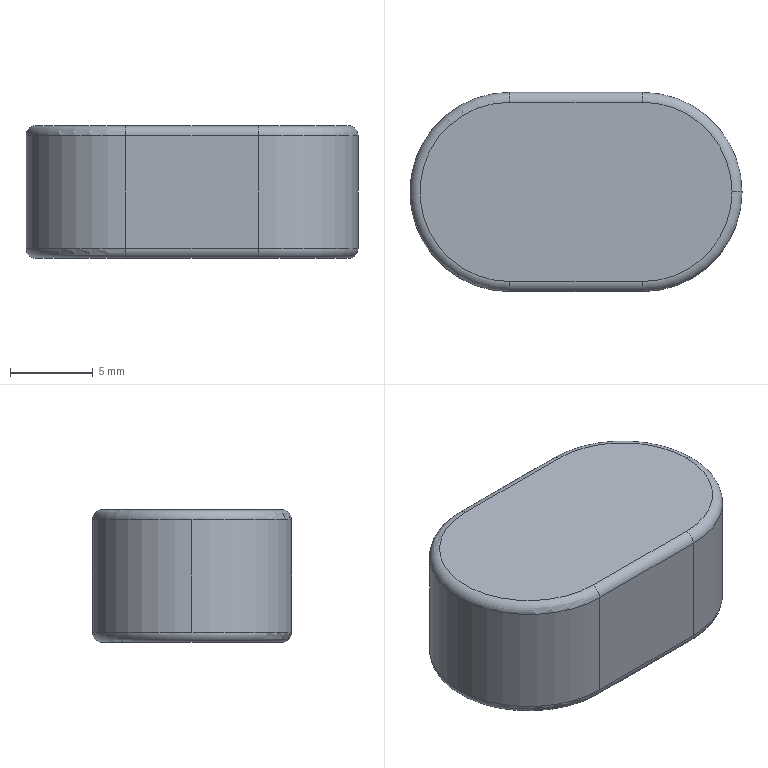Part | SolidWorks | features Extrusion 1, Fillet 1 | 1 solid | 17 faces | box 20 x 12 x 8 mm | volume 1665 mm3 | cylinder 7 | torus 6 | plane 4 | commonest cylinder face diameters 1.2 x4 12 x3
STEP:
#1=CARTESIAN_POINT('',(9.4,0.,0.));
#2=VERTEX_POINT('',#1);
#3=CARTESIAN_POINT('',(4.,-5.4,0.));
#4=VERTEX_POINT('',#3);
#5=CARTESIAN_POINT('',(4.,0.,0.));
#6=DIRECTION('',(0.,0.,-1.));
#7=DIRECTION('',(1.,0.,0.));
#8=AXIS2_PLACEMENT_3D('',#5,#6,#7);
#9=CIRCLE('',#8,5.4);
#10=EDGE_CURVE('',#2,#4,#9,.T.);
#11=ORIENTED_EDGE('',*,*,#10,.F.);
#12=CARTESIAN_POINT('',(10.,0.,0.6));
#13=VERTEX_POINT('',#12);
#14=CARTESIAN_POINT('',(9.4,0.,0.6));
#15=DIRECTION('',(0.,-1.,0.));
#16=DIRECTION('',(0.,0.,-1.));
#17=AXIS2_PLACEMENT_3D('',#14,#15,#16);
#18=CIRCLE('',#17,0.6);
#19=EDGE_CURVE('',#2,#13,#18,.T.);
#20=ORIENTED_EDGE('',*,*,#19,.T.);
#21=CARTESIAN_POINT('',(4.,-6.,0.6));
#22=VERTEX_POINT('',#21);
#23=CARTESIAN_POINT('',(4.,0.,0.6));
#24=DIRECTION('',(0.,0.,1.));
#25=DIRECTION('',(1.,0.,0.));
#26=AXIS2_PLACEMENT_3D('',#23,#24,#25);
#27=CIRCLE('',#26,6.);
#28=EDGE_CURVE('',#22,#13,#27,.T.);
#29=ORIENTED_EDGE('',*,*,#28,.F.);
#30=CARTESIAN_POINT('',(4.,-5.4,0.6));
#31=DIRECTION('',(1.,0.,0.));
#32=DIRECTION('',(0.,0.,-1.));
#33=AXIS2_PLACEMENT_3D('',#30,#31,#32);
#34=CIRCLE('',#33,0.6);
#35=EDGE_CURVE('',#22,#4,#34,.T.);
#36=ORIENTED_EDGE('',*,*,#35,.T.);
#37=EDGE_LOOP('',(#11,#20,#29,#36));
#38=FACE_OUTER_BOUND('',#37,.T.);
#39=CARTESIAN_POINT('',(4.,0.,0.6));
#40=DIRECTION('',(0.,0.,1.));
#41=DIRECTION('',(1.,0.,0.));
#42=AXIS2_PLACEMENT_3D('',#39,#40,#41);
#43=TOROIDAL_SURFACE('',#42,5.4,0.6);
#44=ADVANCED_FACE('',(#38),#43,.T.);
#45=CARTESIAN_POINT('',(10.,0.,7.4));
#46=VERTEX_POINT('',#45);
#47=CARTESIAN_POINT('',(4.,-6.,7.4));
#48=VERTEX_POINT('',#47);
#49=CARTESIAN_POINT('',(4.,0.,7.4));
#50=DIRECTION('',(0.,0.,-1.));
#51=DIRECTION('',(1.,0.,0.));
#52=AXIS2_PLACEMENT_3D('',#49,#50,#51);
#53=CIRCLE('',#52,6.);
#54=EDGE_CURVE('',#46,#48,#53,.T.);
#55=ORIENTED_EDGE('',*,*,#54,.F.);
#56=CARTESIAN_POINT('',(9.4,0.,8.));
#57=VERTEX_POINT('',#56);
#58=CARTESIAN_POINT('',(9.4,0.,7.4));
#59=DIRECTION('',(0.,-1.,0.));
#60=DIRECTION('',(0.,0.,-1.));
#61=AXIS2_PLACEMENT_3D('',#58,#59,#60);
#62=CIRCLE('',#61,0.6);
#63=EDGE_CURVE('',#46,#57,#62,.T.);
#64=ORIENTED_EDGE('',*,*,#63,.T.);
#65=CARTESIAN_POINT('',(4.,-5.4,8.));
#66=VERTEX_POINT('',#65);
#67=CARTESIAN_POINT('',(4.,0.,8.));
#68=DIRECTION('',(0.,0.,1.));
#69=DIRECTION('',(1.,0.,0.));
#70=AXIS2_PLACEMENT_3D('',#67,#68,#69);
#71=CIRCLE('',#70,5.4);
#72=EDGE_CURVE('',#66,#57,#71,.T.);
#73=ORIENTED_EDGE('',*,*,#72,.F.);
#74=CARTESIAN_POINT('',(4.,-5.4,7.4));
#75=DIRECTION('',(1.,0.,0.));
#76=DIRECTION('',(0.,0.,-1.));
#77=AXIS2_PLACEMENT_3D('',#74,#75,#76);
#78=CIRCLE('',#77,0.6);
#79=EDGE_CURVE('',#66,#48,#78,.T.);
#80=ORIENTED_EDGE('',*,*,#79,.T.);
#81=EDGE_LOOP('',(#55,#64,#73,#80));
#82=FACE_OUTER_BOUND('',#81,.T.);
#83=CARTESIAN_POINT('',(4.,0.,7.4));
#84=DIRECTION('',(0.,0.,1.));
#85=DIRECTION('',(1.,0.,0.));
#86=AXIS2_PLACEMENT_3D('',#83,#84,#85);
#87=TOROIDAL_SURFACE('',#86,5.4,0.6);
#88=ADVANCED_FACE('',(#82),#87,.T.);
#89=CARTESIAN_POINT('',(-4.,-6.,7.4));
#90=VERTEX_POINT('',#89);
#91=CARTESIAN_POINT('',(-10.,0.,7.4));
#92=VERTEX_POINT('',#91);
#93=CARTESIAN_POINT('',(-4.,0.,7.4));
#94=DIRECTION('',(0.,0.,-1.));
#95=DIRECTION('',(1.,0.,0.));
#96=AXIS2_PLACEMENT_3D('',#93,#94,#95);
#97=CIRCLE('',#96,6.);
#98=EDGE_CURVE('',#90,#92,#97,.T.);
#99=ORIENTED_EDGE('',*,*,#98,.T.);
#100=CARTESIAN_POINT('',(-10.,0.,0.6));
#101=VERTEX_POINT('',#100);
#102=CARTESIAN_POINT('',(-10.,0.,8.));
#103=DIRECTION('',(0.,0.,-1.));
#104=VECTOR('',#103,1000.);
#105=LINE('',#102,#104);
#106=EDGE_CURVE('',#92,#101,#105,.T.);
#107=ORIENTED_EDGE('',*,*,#106,.T.);
#108=CARTESIAN_POINT('',(-4.,-6.,0.6));
#109=VERTEX_POINT('',#108);
#110=CARTESIAN_POINT('',(-4.,0.,0.6));
#111=DIRECTION('',(0.,0.,1.));
#112=DIRECTION('',(1.,0.,0.));
#113=AXIS2_PLACEMENT_3D('',#110,#111,#112);
#114=CIRCLE('',#113,6.);
#115=EDGE_CURVE('',#101,#109,#114,.T.);
#116=ORIENTED_EDGE('',*,*,#115,.T.);
#117=CARTESIAN_POINT('',(-4.,-6.,8.));
#118=DIRECTION('',(0.,0.,-1.));
#119=VECTOR('',#118,1000.);
#120=LINE('',#117,#119);
#121=EDGE_CURVE('',#90,#109,#120,.T.);
#122=ORIENTED_EDGE('',*,*,#121,.F.);
#123=EDGE_LOOP('',(#99,#107,#116,#122));
#124=FACE_OUTER_BOUND('',#123,.T.);
#125=CARTESIAN_POINT('',(-4.,0.,8.));
#126=DIRECTION('',(0.,0.,-1.));
#127=DIRECTION('',(-1.,0.,0.));
#128=AXIS2_PLACEMENT_3D('',#125,#126,#127);
#129=CYLINDRICAL_SURFACE('',#128,6.);
#130=ADVANCED_FACE('',(#124),#129,.T.);
#131=ORIENTED_EDGE('',*,*,#106,.F.);
#132=CARTESIAN_POINT('',(-4.,6.,7.4));
#133=VERTEX_POINT('',#132);
#134=CARTESIAN_POINT('',(-4.,0.,7.4));
#135=DIRECTION('',(0.,0.,-1.));
#136=DIRECTION('',(1.,0.,0.));
#137=AXIS2_PLACEMENT_3D('',#134,#135,#136);
#138=CIRCLE('',#137,6.);
#139=EDGE_CURVE('',#92,#133,#138,.T.);
#140=ORIENTED_EDGE('',*,*,#139,.T.);
#141=CARTESIAN_POINT('',(-4.,6.,0.6));
#142=VERTEX_POINT('',#141);
#143=CARTESIAN_POINT('',(-4.,6.,8.));
#144=DIRECTION('',(0.,0.,-1.));
#145=VECTOR('',#144,1000.);
#146=LINE('',#143,#145);
#147=EDGE_CURVE('',#133,#142,#146,.T.);
#148=ORIENTED_EDGE('',*,*,#147,.T.);
#149=CARTESIAN_POINT('',(-4.,0.,0.6));
#150=DIRECTION('',(0.,0.,1.));
#151=DIRECTION('',(1.,0.,0.));
#152=AXIS2_PLACEMENT_3D('',#149,#150,#151);
#153=CIRCLE('',#152,6.);
#154=EDGE_CURVE('',#142,#101,#153,.T.);
#155=ORIENTED_EDGE('',*,*,#154,.T.);
#156=EDGE_LOOP('',(#131,#140,#148,#155));
#157=FACE_OUTER_BOUND('',#156,.T.);
#158=CARTESIAN_POINT('',(-4.,0.,8.));
#159=DIRECTION('',(0.,0.,-1.));
#160=DIRECTION('',(-1.,0.,0.));
#161=AXIS2_PLACEMENT_3D('',#158,#159,#160);
#162=CYLINDRICAL_SURFACE('',#161,6.);
#163=ADVANCED_FACE('',(#157),#162,.T.);
#164=CARTESIAN_POINT('',(4.,-6.,8.));
#165=DIRECTION('',(0.,0.,-1.));
#166=VECTOR('',#165,1000.);
#167=LINE('',#164,#166);
#168=EDGE_CURVE('',#48,#22,#167,.T.);
#169=ORIENTED_EDGE('',*,*,#168,.F.);
#170=CARTESIAN_POINT('',(-4.,-6.,7.4));
#171=DIRECTION('',(-1.,0.,0.));
#172=VECTOR('',#171,1000.);
#173=LINE('',#170,#172);
#174=EDGE_CURVE('',#48,#90,#173,.T.);
#175=ORIENTED_EDGE('',*,*,#174,.T.);
#176=ORIENTED_EDGE('',*,*,#121,.T.);
#177=CARTESIAN_POINT('',(-4.,-6.,0.6));
#178=DIRECTION('',(1.,0.,0.));
#179=VECTOR('',#178,1000.);
#180=LINE('',#177,#179);
#181=EDGE_CURVE('',#109,#22,#180,.T.);
#182=ORIENTED_EDGE('',*,*,#181,.T.);
#183=EDGE_LOOP('',(#169,#175,#176,#182));
#184=FACE_OUTER_BOUND('',#183,.T.);
#185=CARTESIAN_POINT('',(-4.,-6.,8.));
#186=DIRECTION('',(0.,1.,0.));
#187=DIRECTION('',(-1.,0.,0.));
#188=AXIS2_PLACEMENT_3D('',#185,#186,#187);
#189=PLANE('',#188);
#190=ADVANCED_FACE('',(#184),#189,.F.);
#191=CARTESIAN_POINT('',(4.,6.,7.4));
#192=VERTEX_POINT('',#191);
#193=CARTESIAN_POINT('',(4.,6.,0.6));
#194=VERTEX_POINT('',#193);
#195=CARTESIAN_POINT('',(4.,6.,8.));
#196=DIRECTION('',(0.,0.,-1.));
#197=VECTOR('',#196,1000.);
#198=LINE('',#195,#197);
#199=EDGE_CURVE('',#192,#194,#198,.T.);
#200=ORIENTED_EDGE('',*,*,#199,.F.);
#201=CARTESIAN_POINT('',(4.,0.,7.4));
#202=DIRECTION('',(0.,0.,-1.));
#203=DIRECTION('',(1.,0.,0.));
#204=AXIS2_PLACEMENT_3D('',#201,#202,#203);
#205=CIRCLE('',#204,6.);
#206=EDGE_CURVE('',#192,#46,#205,.T.);
#207=ORIENTED_EDGE('',*,*,#206,.T.);
#208=ORIENTED_EDGE('',*,*,#54,.T.);
#209=ORIENTED_EDGE('',*,*,#168,.T.);
#210=ORIENTED_EDGE('',*,*,#28,.T.);
#211=CARTESIAN_POINT('',(4.,0.,0.6));
#212=DIRECTION('',(0.,0.,1.));
#213=DIRECTION('',(1.,0.,0.));
#214=AXIS2_PLACEMENT_3D('',#211,#212,#213);
#215=CIRCLE('',#214,6.);
#216=EDGE_CURVE('',#13,#194,#215,.T.);
#217=ORIENTED_EDGE('',*,*,#216,.T.);
#218=EDGE_LOOP('',(#200,#207,#208,#209,#210,#217));
#219=FACE_OUTER_BOUND('',#218,.T.);
#220=CARTESIAN_POINT('',(4.,0.,8.));
#221=DIRECTION('',(0.,0.,-1.));
#222=DIRECTION('',(-1.,0.,0.));
#223=AXIS2_PLACEMENT_3D('',#220,#221,#222);
#224=CYLINDRICAL_SURFACE('',#223,6.);
#225=ADVANCED_FACE('',(#219),#224,.T.);
#226=ORIENTED_EDGE('',*,*,#147,.F.);
#227=CARTESIAN_POINT('',(4.,6.,7.4));
#228=DIRECTION('',(1.,0.,0.));
#229=VECTOR('',#228,1000.);
#230=LINE('',#227,#229);
#231=EDGE_CURVE('',#133,#192,#230,.T.);
#232=ORIENTED_EDGE('',*,*,#231,.T.);
#233=ORIENTED_EDGE('',*,*,#199,.T.);
#234=CARTESIAN_POINT('',(-4.,6.,0.6));
#235=DIRECTION('',(-1.,0.,0.));
#236=VECTOR('',#235,1000.);
#237=LINE('',#234,#236);
#238=EDGE_CURVE('',#194,#142,#237,.T.);
#239=ORIENTED_EDGE('',*,*,#238,.T.);
#240=EDGE_LOOP('',(#226,#232,#233,#239));
#241=FACE_OUTER_BOUND('',#240,.T.);
#242=CARTESIAN_POINT('',(-4.,6.,8.));
#243=DIRECTION('',(0.,-1.,0.));
#244=DIRECTION('',(1.,0.,0.));
#245=AXIS2_PLACEMENT_3D('',#242,#243,#244);
#246=PLANE('',#245);
#247=ADVANCED_FACE('',(#241),#246,.F.);
#248=CARTESIAN_POINT('',(-4.,-5.4,8.));
#249=VERTEX_POINT('',#248);
#250=CARTESIAN_POINT('',(4.,-5.4,8.));
#251=DIRECTION('',(1.,0.,0.));
#252=VECTOR('',#251,1000.);
#253=LINE('',#250,#252);
#254=EDGE_CURVE('',#249,#66,#253,.T.);
#255=ORIENTED_EDGE('',*,*,#254,.T.);
#256=ORIENTED_EDGE('',*,*,#72,.T.);
#257=CARTESIAN_POINT('',(4.,5.4,8.));
#258=VERTEX_POINT('',#257);
#259=CARTESIAN_POINT('',(4.,0.,8.));
#260=DIRECTION('',(0.,0.,1.));
#261=DIRECTION('',(1.,0.,0.));
#262=AXIS2_PLACEMENT_3D('',#259,#260,#261);
#263=CIRCLE('',#262,5.4);
#264=EDGE_CURVE('',#57,#258,#263,.T.);
#265=ORIENTED_EDGE('',*,*,#264,.T.);
#266=CARTESIAN_POINT('',(-4.,5.4,8.));
#267=VERTEX_POINT('',#266);
#268=CARTESIAN_POINT('',(-4.,5.4,8.));
#269=DIRECTION('',(-1.,0.,0.));
#270=VECTOR('',#269,1000.);
#271=LINE('',#268,#270);
#272=EDGE_CURVE('',#258,#267,#271,.T.);
#273=ORIENTED_EDGE('',*,*,#272,.T.);
#274=CARTESIAN_POINT('',(-4.,0.,8.));
#275=DIRECTION('',(0.,0.,1.));
#276=DIRECTION('',(1.,0.,0.));
#277=AXIS2_PLACEMENT_3D('',#274,#275,#276);
#278=CIRCLE('',#277,5.4);
#279=EDGE_CURVE('',#267,#249,#278,.T.);
#280=ORIENTED_EDGE('',*,*,#279,.T.);
#281=EDGE_LOOP('',(#255,#256,#265,#273,#280));
#282=FACE_OUTER_BOUND('',#281,.T.);
#283=CARTESIAN_POINT('',(-4.,0.,8.));
#284=DIRECTION('',(0.,0.,1.));
#285=DIRECTION('',(1.,0.,0.));
#286=AXIS2_PLACEMENT_3D('',#283,#284,#285);
#287=PLANE('',#286);
#288=ADVANCED_FACE('',(#282),#287,.T.);
#289=CARTESIAN_POINT('',(-4.,5.4,0.));
#290=VERTEX_POINT('',#289);
#291=CARTESIAN_POINT('',(4.,5.4,0.));
#292=VERTEX_POINT('',#291);
#293=CARTESIAN_POINT('',(-4.,5.4,0.));
#294=DIRECTION('',(1.,0.,0.));
#295=VECTOR('',#294,1000.);
#296=LINE('',#293,#295);
#297=EDGE_CURVE('',#290,#292,#296,.T.);
#298=ORIENTED_EDGE('',*,*,#297,.T.);
#299=CARTESIAN_POINT('',(4.,0.,0.));
#300=DIRECTION('',(0.,0.,-1.));
#301=DIRECTION('',(1.,0.,0.));
#302=AXIS2_PLACEMENT_3D('',#299,#300,#301);
#303=CIRCLE('',#302,5.4);
#304=EDGE_CURVE('',#292,#2,#303,.T.);
#305=ORIENTED_EDGE('',*,*,#304,.T.);
#306=ORIENTED_EDGE('',*,*,#10,.T.);
#307=CARTESIAN_POINT('',(-4.,-5.4,0.));
#308=VERTEX_POINT('',#307);
#309=CARTESIAN_POINT('',(-4.,-5.4,0.));
#310=DIRECTION('',(-1.,0.,0.));
#311=VECTOR('',#310,1000.);
#312=LINE('',#309,#311);
#313=EDGE_CURVE('',#4,#308,#312,.T.);
#314=ORIENTED_EDGE('',*,*,#313,.T.);
#315=CARTESIAN_POINT('',(-4.,0.,0.));
#316=DIRECTION('',(0.,0.,-1.));
#317=DIRECTION('',(1.,0.,0.));
#318=AXIS2_PLACEMENT_3D('',#315,#316,#317);
#319=CIRCLE('',#318,5.4);
#320=EDGE_CURVE('',#308,#290,#319,.T.);
#321=ORIENTED_EDGE('',*,*,#320,.T.);
#322=EDGE_LOOP('',(#298,#305,#306,#314,#321));
#323=FACE_OUTER_BOUND('',#322,.T.);
#324=CARTESIAN_POINT('',(-4.,0.,0.));
#325=DIRECTION('',(0.,0.,1.));
#326=DIRECTION('',(1.,0.,0.));
#327=AXIS2_PLACEMENT_3D('',#324,#325,#326);
#328=PLANE('',#327);
#329=ADVANCED_FACE('',(#323),#328,.F.);
#330=CARTESIAN_POINT('',(-4.,5.4,7.4));
#331=DIRECTION('',(1.,0.,0.));
#332=DIRECTION('',(0.,0.,-1.));
#333=AXIS2_PLACEMENT_3D('',#330,#331,#332);
#334=CIRCLE('',#333,0.6);
#335=EDGE_CURVE('',#133,#267,#334,.T.);
#336=ORIENTED_EDGE('',*,*,#335,.F.);
#337=ORIENTED_EDGE('',*,*,#139,.F.);
#338=ORIENTED_EDGE('',*,*,#98,.F.);
#339=CARTESIAN_POINT('',(-4.,-5.4,7.4));
#340=DIRECTION('',(1.,0.,0.));
#341=DIRECTION('',(0.,0.,-1.));
#342=AXIS2_PLACEMENT_3D('',#339,#340,#341);
#343=CIRCLE('',#342,0.6);
#344=EDGE_CURVE('',#249,#90,#343,.T.);
#345=ORIENTED_EDGE('',*,*,#344,.F.);
#346=ORIENTED_EDGE('',*,*,#279,.F.);
#347=EDGE_LOOP('',(#336,#337,#338,#345,#346));
#348=FACE_OUTER_BOUND('',#347,.T.);
#349=CARTESIAN_POINT('',(-4.,0.,7.4));
#350=DIRECTION('',(0.,0.,1.));
#351=DIRECTION('',(1.,0.,0.));
#352=AXIS2_PLACEMENT_3D('',#349,#350,#351);
#353=TOROIDAL_SURFACE('',#352,5.4,0.6);
#354=ADVANCED_FACE('',(#348),#353,.T.);
#355=ORIENTED_EDGE('',*,*,#344,.T.);
#356=ORIENTED_EDGE('',*,*,#174,.F.);
#357=ORIENTED_EDGE('',*,*,#79,.F.);
#358=ORIENTED_EDGE('',*,*,#254,.F.);
#359=EDGE_LOOP('',(#355,#356,#357,#358));
#360=FACE_OUTER_BOUND('',#359,.T.);
#361=CARTESIAN_POINT('',(-4.,-5.4,7.4));
#362=DIRECTION('',(-1.,0.,0.));
#363=DIRECTION('',(0.,-1.,0.));
#364=AXIS2_PLACEMENT_3D('',#361,#362,#363);
#365=CYLINDRICAL_SURFACE('',#364,0.6);
#366=ADVANCED_FACE('',(#360),#365,.T.);
#367=ORIENTED_EDGE('',*,*,#335,.T.);
#368=ORIENTED_EDGE('',*,*,#272,.F.);
#369=CARTESIAN_POINT('',(4.,5.4,7.4));
#370=DIRECTION('',(1.,0.,0.));
#371=DIRECTION('',(0.,0.,-1.));
#372=AXIS2_PLACEMENT_3D('',#369,#370,#371);
#373=CIRCLE('',#372,0.6);
#374=EDGE_CURVE('',#192,#258,#373,.T.);
#375=ORIENTED_EDGE('',*,*,#374,.F.);
#376=ORIENTED_EDGE('',*,*,#231,.F.);
#377=EDGE_LOOP('',(#367,#368,#375,#376));
#378=FACE_OUTER_BOUND('',#377,.T.);
#379=CARTESIAN_POINT('',(-4.,5.4,7.4));
#380=DIRECTION('',(1.,0.,0.));
#381=DIRECTION('',(0.,1.,0.));
#382=AXIS2_PLACEMENT_3D('',#379,#380,#381);
#383=CYLINDRICAL_SURFACE('',#382,0.6);
#384=ADVANCED_FACE('',(#378),#383,.T.);
#385=ORIENTED_EDGE('',*,*,#63,.F.);
#386=ORIENTED_EDGE('',*,*,#206,.F.);
#387=ORIENTED_EDGE('',*,*,#374,.T.);
#388=ORIENTED_EDGE('',*,*,#264,.F.);
#389=EDGE_LOOP('',(#385,#386,#387,#388));
#390=FACE_OUTER_BOUND('',#389,.T.);
#391=CARTESIAN_POINT('',(4.,0.,7.4));
#392=DIRECTION('',(0.,0.,1.));
#393=DIRECTION('',(1.,0.,0.));
#394=AXIS2_PLACEMENT_3D('',#391,#392,#393);
#395=TOROIDAL_SURFACE('',#394,5.4,0.6);
#396=ADVANCED_FACE('',(#390),#395,.T.);
#397=CARTESIAN_POINT('',(-4.,5.4,0.6));
#398=DIRECTION('',(1.,0.,0.));
#399=DIRECTION('',(0.,0.,-1.));
#400=AXIS2_PLACEMENT_3D('',#397,#398,#399);
#401=CIRCLE('',#400,0.6);
#402=EDGE_CURVE('',#290,#142,#401,.T.);
#403=ORIENTED_EDGE('',*,*,#402,.F.);
#404=ORIENTED_EDGE('',*,*,#320,.F.);
#405=CARTESIAN_POINT('',(-4.,-5.4,0.6));
#406=DIRECTION('',(1.,0.,0.));
#407=DIRECTION('',(0.,0.,-1.));
#408=AXIS2_PLACEMENT_3D('',#405,#406,#407);
#409=CIRCLE('',#408,0.6);
#410=EDGE_CURVE('',#109,#308,#409,.T.);
#411=ORIENTED_EDGE('',*,*,#410,.F.);
#412=ORIENTED_EDGE('',*,*,#115,.F.);
#413=ORIENTED_EDGE('',*,*,#154,.F.);
#414=EDGE_LOOP('',(#403,#404,#411,#412,#413));
#415=FACE_OUTER_BOUND('',#414,.T.);
#416=CARTESIAN_POINT('',(-4.,0.,0.6));
#417=DIRECTION('',(0.,0.,1.));
#418=DIRECTION('',(1.,0.,0.));
#419=AXIS2_PLACEMENT_3D('',#416,#417,#418);
#420=TOROIDAL_SURFACE('',#419,5.4,0.6);
#421=ADVANCED_FACE('',(#415),#420,.T.);
#422=ORIENTED_EDGE('',*,*,#410,.T.);
#423=ORIENTED_EDGE('',*,*,#313,.F.);
#424=ORIENTED_EDGE('',*,*,#35,.F.);
#425=ORIENTED_EDGE('',*,*,#181,.F.);
#426=EDGE_LOOP('',(#422,#423,#424,#425));
#427=FACE_OUTER_BOUND('',#426,.T.);
#428=CARTESIAN_POINT('',(-4.,-5.4,0.6));
#429=DIRECTION('',(1.,0.,0.));
#430=DIRECTION('',(0.,1.,0.));
#431=AXIS2_PLACEMENT_3D('',#428,#429,#430);
#432=CYLINDRICAL_SURFACE('',#431,0.6);
#433=ADVANCED_FACE('',(#427),#432,.T.);
#434=ORIENTED_EDGE('',*,*,#402,.T.);
#435=ORIENTED_EDGE('',*,*,#238,.F.);
#436=CARTESIAN_POINT('',(4.,5.4,0.6));
#437=DIRECTION('',(1.,0.,0.));
#438=DIRECTION('',(0.,0.,-1.));
#439=AXIS2_PLACEMENT_3D('',#436,#437,#438);
#440=CIRCLE('',#439,0.6);
#441=EDGE_CURVE('',#292,#194,#440,.T.);
#442=ORIENTED_EDGE('',*,*,#441,.F.);
#443=ORIENTED_EDGE('',*,*,#297,.F.);
#444=EDGE_LOOP('',(#434,#435,#442,#443));
#445=FACE_OUTER_BOUND('',#444,.T.);
#446=CARTESIAN_POINT('',(-4.,5.4,0.6));
#447=DIRECTION('',(-1.,0.,0.));
#448=DIRECTION('',(0.,-1.,0.));
#449=AXIS2_PLACEMENT_3D('',#446,#447,#448);
#450=CYLINDRICAL_SURFACE('',#449,0.6);
#451=ADVANCED_FACE('',(#445),#450,.T.);
#452=ORIENTED_EDGE('',*,*,#19,.F.);
#453=ORIENTED_EDGE('',*,*,#304,.F.);
#454=ORIENTED_EDGE('',*,*,#441,.T.);
#455=ORIENTED_EDGE('',*,*,#216,.F.);
#456=EDGE_LOOP('',(#452,#453,#454,#455));
#457=FACE_OUTER_BOUND('',#456,.T.);
#458=CARTESIAN_POINT('',(4.,0.,0.6));
#459=DIRECTION('',(0.,0.,1.));
#460=DIRECTION('',(1.,0.,0.));
#461=AXIS2_PLACEMENT_3D('',#458,#459,#460);
#462=TOROIDAL_SURFACE('',#461,5.4,0.6);
#463=ADVANCED_FACE('',(#457),#462,.T.);
#464=CLOSED_SHELL('',(#44,#88,#130,#163,#190,#225,#247,#288,#329,#354,#366,#384,#396,#421,#433,#451,#463));
#465=MANIFOLD_SOLID_BREP('',#464);
#466=CARTESIAN_POINT('',(0.,0.,0.));
#467=DIRECTION('',(0.,0.,1.));
#468=DIRECTION('',(1.,0.,0.));
#469=AXIS2_PLACEMENT_3D('',#466,#467,#468);
#470=(LENGTH_UNIT()NAMED_UNIT(*)SI_UNIT(.MILLI.,.METRE.));
#471=UNCERTAINTY_MEASURE_WITH_UNIT(LENGTH_MEASURE(0.00001),#470,'','');
#472=(NAMED_UNIT(*)PLANE_ANGLE_UNIT()SI_UNIT($,.RADIAN.));
#473=(NAMED_UNIT(*)SI_UNIT($,.STERADIAN.)SOLID_ANGLE_UNIT());
#474=(GEOMETRIC_REPRESENTATION_CONTEXT(3)GLOBAL_UNCERTAINTY_ASSIGNED_CONTEXT((#471))GLOBAL_UNIT_ASSIGNED_CONTEXT((#470,#472,#473))REPRESENTATION_CONTEXT('',''));
#475=ADVANCED_BREP_SHAPE_REPRESENTATION('',(#465,#469),#474);